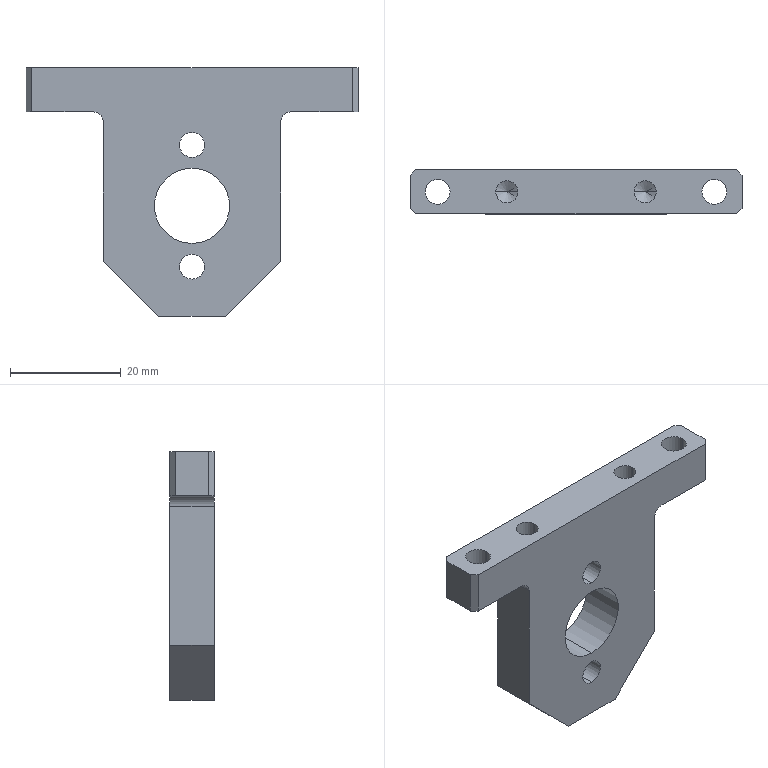Part | SolidWorks | features HoleWzd 3, Chamfer 2, Extrusion 1, ICE 1 | 1 solid | 42 faces | box 60 x 8 x 45 mm | volume 10317 mm3 | cylinder 20 | plane 18 | cone 4 | commonest cylinder face diameters 4.5 x8 4 x6 7.5 x4 13.6 x2
STEP:
#1=CARTESIAN_POINT('',(27.25,0.,0.));
#2=VERTEX_POINT('',#1);
#3=CARTESIAN_POINT('',(22.75,0.,0.));
#4=VERTEX_POINT('',#3);
#5=CARTESIAN_POINT('',(25.,0.,0.));
#6=DIRECTION('',(0.,0.,-1.));
#7=DIRECTION('',(-1.,0.,0.));
#8=AXIS2_PLACEMENT_3D('',#5,#6,#7);
#9=CIRCLE('',#8,2.25);
#10=EDGE_CURVE('',#2,#4,#9,.T.);
#11=ORIENTED_EDGE('',*,*,#10,.F.);
#12=CARTESIAN_POINT('',(27.25,0.,-8.));
#13=VERTEX_POINT('',#12);
#14=CARTESIAN_POINT('',(27.25,0.,-8.));
#15=DIRECTION('',(0.,0.,-1.));
#16=VECTOR('',#15,1000.);
#17=LINE('',#14,#16);
#18=EDGE_CURVE('',#2,#13,#17,.T.);
#19=ORIENTED_EDGE('',*,*,#18,.T.);
#20=CARTESIAN_POINT('',(22.75,0.,-8.));
#21=VERTEX_POINT('',#20);
#22=CARTESIAN_POINT('',(25.,0.,-8.));
#23=DIRECTION('',(0.,0.,-1.));
#24=DIRECTION('',(-1.,0.,0.));
#25=AXIS2_PLACEMENT_3D('',#22,#23,#24);
#26=CIRCLE('',#25,2.25);
#27=EDGE_CURVE('',#13,#21,#26,.T.);
#28=ORIENTED_EDGE('',*,*,#27,.T.);
#29=CARTESIAN_POINT('',(22.75,0.,-8.));
#30=DIRECTION('',(0.,0.,-1.));
#31=VECTOR('',#30,1000.);
#32=LINE('',#29,#31);
#33=EDGE_CURVE('',#4,#21,#32,.T.);
#34=ORIENTED_EDGE('',*,*,#33,.F.);
#35=EDGE_LOOP('',(#11,#19,#28,#34));
#36=FACE_OUTER_BOUND('',#35,.T.);
#37=CARTESIAN_POINT('',(25.,0.,-8.));
#38=DIRECTION('',(0.,0.,-1.));
#39=DIRECTION('',(-1.,0.,0.));
#40=AXIS2_PLACEMENT_3D('',#37,#38,#39);
#41=CYLINDRICAL_SURFACE('',#40,2.25);
#42=ADVANCED_FACE('',(#36),#41,.F.);
#43=CARTESIAN_POINT('',(-22.75,0.,0.));
#44=VERTEX_POINT('',#43);
#45=CARTESIAN_POINT('',(-27.25,0.,0.));
#46=VERTEX_POINT('',#45);
#47=CARTESIAN_POINT('',(-25.,0.,0.));
#48=DIRECTION('',(0.,0.,-1.));
#49=DIRECTION('',(-1.,0.,0.));
#50=AXIS2_PLACEMENT_3D('',#47,#48,#49);
#51=CIRCLE('',#50,2.25);
#52=EDGE_CURVE('',#44,#46,#51,.T.);
#53=ORIENTED_EDGE('',*,*,#52,.F.);
#54=CARTESIAN_POINT('',(-22.75,0.,-8.));
#55=VERTEX_POINT('',#54);
#56=CARTESIAN_POINT('',(-22.75,0.,-8.));
#57=DIRECTION('',(0.,0.,-1.));
#58=VECTOR('',#57,1000.);
#59=LINE('',#56,#58);
#60=EDGE_CURVE('',#44,#55,#59,.T.);
#61=ORIENTED_EDGE('',*,*,#60,.T.);
#62=CARTESIAN_POINT('',(-27.25,0.,-8.));
#63=VERTEX_POINT('',#62);
#64=CARTESIAN_POINT('',(-25.,0.,-8.));
#65=DIRECTION('',(0.,0.,-1.));
#66=DIRECTION('',(-1.,0.,0.));
#67=AXIS2_PLACEMENT_3D('',#64,#65,#66);
#68=CIRCLE('',#67,2.25);
#69=EDGE_CURVE('',#55,#63,#68,.T.);
#70=ORIENTED_EDGE('',*,*,#69,.T.);
#71=CARTESIAN_POINT('',(-27.25,0.,-8.));
#72=DIRECTION('',(0.,0.,-1.));
#73=VECTOR('',#72,1000.);
#74=LINE('',#71,#73);
#75=EDGE_CURVE('',#46,#63,#74,.T.);
#76=ORIENTED_EDGE('',*,*,#75,.F.);
#77=EDGE_LOOP('',(#53,#61,#70,#76));
#78=FACE_OUTER_BOUND('',#77,.T.);
#79=CARTESIAN_POINT('',(-25.,0.,-8.));
#80=DIRECTION('',(0.,0.,-1.));
#81=DIRECTION('',(-1.,0.,0.));
#82=AXIS2_PLACEMENT_3D('',#79,#80,#81);
#83=CYLINDRICAL_SURFACE('',#82,2.25);
#84=ADVANCED_FACE('',(#78),#83,.F.);
#85=CARTESIAN_POINT('',(-14.5,0.,-10.));
#86=VERTEX_POINT('',#85);
#87=CARTESIAN_POINT('',(-10.5,0.,-10.));
#88=VERTEX_POINT('',#87);
#89=CARTESIAN_POINT('',(-12.5,0.,-10.));
#90=DIRECTION('',(0.,0.,1.));
#91=DIRECTION('',(1.,0.,0.));
#92=AXIS2_PLACEMENT_3D('',#89,#90,#91);
#93=CIRCLE('',#92,2.);
#94=EDGE_CURVE('',#86,#88,#93,.T.);
#95=ORIENTED_EDGE('',*,*,#94,.F.);
#96=CARTESIAN_POINT('',(-14.5,0.,0.));
#97=VERTEX_POINT('',#96);
#98=CARTESIAN_POINT('',(-14.5,0.,0.));
#99=DIRECTION('',(0.,0.,1.));
#100=VECTOR('',#99,1000.);
#101=LINE('',#98,#100);
#102=EDGE_CURVE('',#86,#97,#101,.T.);
#103=ORIENTED_EDGE('',*,*,#102,.T.);
#104=CARTESIAN_POINT('',(-10.5,0.,0.));
#105=VERTEX_POINT('',#104);
#106=CARTESIAN_POINT('',(-12.5,0.,0.));
#107=DIRECTION('',(0.,0.,1.));
#108=DIRECTION('',(1.,0.,0.));
#109=AXIS2_PLACEMENT_3D('',#106,#107,#108);
#110=CIRCLE('',#109,2.);
#111=EDGE_CURVE('',#97,#105,#110,.T.);
#112=ORIENTED_EDGE('',*,*,#111,.T.);
#113=CARTESIAN_POINT('',(-10.5,0.,0.));
#114=DIRECTION('',(0.,0.,1.));
#115=VECTOR('',#114,1000.);
#116=LINE('',#113,#115);
#117=EDGE_CURVE('',#88,#105,#116,.T.);
#118=ORIENTED_EDGE('',*,*,#117,.F.);
#119=EDGE_LOOP('',(#95,#103,#112,#118));
#120=FACE_OUTER_BOUND('',#119,.T.);
#121=CARTESIAN_POINT('',(-12.5,0.,0.));
#122=DIRECTION('',(0.,0.,1.));
#123=DIRECTION('',(1.,0.,0.));
#124=AXIS2_PLACEMENT_3D('',#121,#122,#123);
#125=CYLINDRICAL_SURFACE('',#124,2.);
#126=ADVANCED_FACE('',(#120),#125,.F.);
#127=CARTESIAN_POINT('',(-12.5,0.,-11.202));
#128=VERTEX_POINT('',#127);
#129=CARTESIAN_POINT('',(-10.5,0.,-10.));
#130=DIRECTION('',(0.8572,0.,0.515));
#131=VECTOR('',#130,1000.);
#132=LINE('',#129,#131);
#133=EDGE_CURVE('',#128,#88,#132,.T.);
#134=ORIENTED_EDGE('',*,*,#133,.F.);
#135=CARTESIAN_POINT('',(-14.5,0.,-10.));
#136=DIRECTION('',(-0.8572,0.,0.515));
#137=VECTOR('',#136,1000.);
#138=LINE('',#135,#137);
#139=EDGE_CURVE('',#128,#86,#138,.T.);
#140=ORIENTED_EDGE('',*,*,#139,.T.);
#141=ORIENTED_EDGE('',*,*,#94,.T.);
#142=EDGE_LOOP('',(#134,#140,#141));
#143=FACE_OUTER_BOUND('',#142,.T.);
#144=CARTESIAN_POINT('',(-12.5,0.,-10.));
#145=DIRECTION('',(0.,0.,1.));
#146=DIRECTION('',(1.,0.,0.));
#147=AXIS2_PLACEMENT_3D('',#144,#145,#146);
#148=CONICAL_SURFACE('',#147,2.,1.03);
#149=ADVANCED_FACE('',(#143),#148,.F.);
#150=CARTESIAN_POINT('',(10.5,0.,-10.));
#151=VERTEX_POINT('',#150);
#152=CARTESIAN_POINT('',(14.5,0.,-10.));
#153=VERTEX_POINT('',#152);
#154=CARTESIAN_POINT('',(12.5,0.,-10.));
#155=DIRECTION('',(0.,0.,1.));
#156=DIRECTION('',(1.,0.,0.));
#157=AXIS2_PLACEMENT_3D('',#154,#155,#156);
#158=CIRCLE('',#157,2.);
#159=EDGE_CURVE('',#151,#153,#158,.T.);
#160=ORIENTED_EDGE('',*,*,#159,.F.);
#161=CARTESIAN_POINT('',(10.5,0.,0.));
#162=VERTEX_POINT('',#161);
#163=CARTESIAN_POINT('',(10.5,0.,0.));
#164=DIRECTION('',(0.,0.,1.));
#165=VECTOR('',#164,1000.);
#166=LINE('',#163,#165);
#167=EDGE_CURVE('',#151,#162,#166,.T.);
#168=ORIENTED_EDGE('',*,*,#167,.T.);
#169=CARTESIAN_POINT('',(14.5,0.,0.));
#170=VERTEX_POINT('',#169);
#171=CARTESIAN_POINT('',(12.5,0.,0.));
#172=DIRECTION('',(0.,0.,1.));
#173=DIRECTION('',(1.,0.,0.));
#174=AXIS2_PLACEMENT_3D('',#171,#172,#173);
#175=CIRCLE('',#174,2.);
#176=EDGE_CURVE('',#162,#170,#175,.T.);
#177=ORIENTED_EDGE('',*,*,#176,.T.);
#178=CARTESIAN_POINT('',(14.5,0.,0.));
#179=DIRECTION('',(0.,0.,1.));
#180=VECTOR('',#179,1000.);
#181=LINE('',#178,#180);
#182=EDGE_CURVE('',#153,#170,#181,.T.);
#183=ORIENTED_EDGE('',*,*,#182,.F.);
#184=EDGE_LOOP('',(#160,#168,#177,#183));
#185=FACE_OUTER_BOUND('',#184,.T.);
#186=CARTESIAN_POINT('',(12.5,0.,0.));
#187=DIRECTION('',(0.,0.,1.));
#188=DIRECTION('',(1.,0.,0.));
#189=AXIS2_PLACEMENT_3D('',#186,#187,#188);
#190=CYLINDRICAL_SURFACE('',#189,2.);
#191=ADVANCED_FACE('',(#185),#190,.F.);
#192=CARTESIAN_POINT('',(12.5,0.,-11.202));
#193=VERTEX_POINT('',#192);
#194=CARTESIAN_POINT('',(14.5,0.,-10.));
#195=DIRECTION('',(0.8572,0.,0.515));
#196=VECTOR('',#195,1000.);
#197=LINE('',#194,#196);
#198=EDGE_CURVE('',#193,#153,#197,.T.);
#199=ORIENTED_EDGE('',*,*,#198,.F.);
#200=CARTESIAN_POINT('',(10.5,0.,-10.));
#201=DIRECTION('',(-0.8572,0.,0.515));
#202=VECTOR('',#201,1000.);
#203=LINE('',#200,#202);
#204=EDGE_CURVE('',#193,#151,#203,.T.);
#205=ORIENTED_EDGE('',*,*,#204,.T.);
#206=ORIENTED_EDGE('',*,*,#159,.T.);
#207=EDGE_LOOP('',(#199,#205,#206));
#208=FACE_OUTER_BOUND('',#207,.T.);
#209=CARTESIAN_POINT('',(12.5,0.,-10.));
#210=DIRECTION('',(0.,0.,1.));
#211=DIRECTION('',(1.,0.,0.));
#212=AXIS2_PLACEMENT_3D('',#209,#210,#211);
#213=CONICAL_SURFACE('',#212,2.,1.03);
#214=ADVANCED_FACE('',(#208),#213,.F.);
#215=CARTESIAN_POINT('',(0.,-0.6,-39.75));
#216=VERTEX_POINT('',#215);
#217=CARTESIAN_POINT('',(0.,-0.6,-32.25));
#218=VERTEX_POINT('',#217);
#219=CARTESIAN_POINT('',(0.,-0.6,-36.));
#220=DIRECTION('',(0.,1.,0.));
#221=DIRECTION('',(0.,0.,1.));
#222=AXIS2_PLACEMENT_3D('',#219,#220,#221);
#223=CIRCLE('',#222,3.75);
#224=EDGE_CURVE('',#216,#218,#223,.T.);
#225=ORIENTED_EDGE('',*,*,#224,.F.);
#226=CARTESIAN_POINT('',(0.,4.,-39.75));
#227=VERTEX_POINT('',#226);
#228=CARTESIAN_POINT('',(0.,4.,-39.75));
#229=DIRECTION('',(0.,1.,0.));
#230=VECTOR('',#229,1000.);
#231=LINE('',#228,#230);
#232=EDGE_CURVE('',#216,#227,#231,.T.);
#233=ORIENTED_EDGE('',*,*,#232,.T.);
#234=CARTESIAN_POINT('',(0.,4.,-32.25));
#235=VERTEX_POINT('',#234);
#236=CARTESIAN_POINT('',(0.,4.,-36.));
#237=DIRECTION('',(0.,1.,0.));
#238=DIRECTION('',(0.,0.,1.));
#239=AXIS2_PLACEMENT_3D('',#236,#237,#238);
#240=CIRCLE('',#239,3.75);
#241=EDGE_CURVE('',#227,#235,#240,.T.);
#242=ORIENTED_EDGE('',*,*,#241,.T.);
#243=CARTESIAN_POINT('',(0.,4.,-32.25));
#244=DIRECTION('',(0.,1.,0.));
#245=VECTOR('',#244,1000.);
#246=LINE('',#243,#245);
#247=EDGE_CURVE('',#218,#235,#246,.T.);
#248=ORIENTED_EDGE('',*,*,#247,.F.);
#249=EDGE_LOOP('',(#225,#233,#242,#248));
#250=FACE_OUTER_BOUND('',#249,.T.);
#251=CARTESIAN_POINT('',(0.,4.,-36.));
#252=DIRECTION('',(0.,1.,0.));
#253=DIRECTION('',(0.,0.,1.));
#254=AXIS2_PLACEMENT_3D('',#251,#252,#253);
#255=CYLINDRICAL_SURFACE('',#254,3.75);
#256=ADVANCED_FACE('',(#250),#255,.F.);
#257=CARTESIAN_POINT('',(0.,-4.,-33.75));
#258=VERTEX_POINT('',#257);
#259=CARTESIAN_POINT('',(0.,-4.,-38.25));
#260=VERTEX_POINT('',#259);
#261=CARTESIAN_POINT('',(0.,-4.,-36.));
#262=DIRECTION('',(0.,-1.,0.));
#263=DIRECTION('',(0.,0.,-1.));
#264=AXIS2_PLACEMENT_3D('',#261,#262,#263);
#265=CIRCLE('',#264,2.25);
#266=EDGE_CURVE('',#258,#260,#265,.T.);
#267=ORIENTED_EDGE('',*,*,#266,.T.);
#268=CARTESIAN_POINT('',(0.,-0.6,-38.25));
#269=VERTEX_POINT('',#268);
#270=CARTESIAN_POINT('',(0.,4.,-38.25));
#271=DIRECTION('',(0.,1.,0.));
#272=VECTOR('',#271,1000.);
#273=LINE('',#270,#272);
#274=EDGE_CURVE('',#260,#269,#273,.T.);
#275=ORIENTED_EDGE('',*,*,#274,.T.);
#276=CARTESIAN_POINT('',(0.,-0.6,-33.75));
#277=VERTEX_POINT('',#276);
#278=CARTESIAN_POINT('',(0.,-0.6,-36.));
#279=DIRECTION('',(0.,1.,0.));
#280=DIRECTION('',(0.,0.,1.));
#281=AXIS2_PLACEMENT_3D('',#278,#279,#280);
#282=CIRCLE('',#281,2.25);
#283=EDGE_CURVE('',#269,#277,#282,.T.);
#284=ORIENTED_EDGE('',*,*,#283,.T.);
#285=CARTESIAN_POINT('',(0.,4.,-33.75));
#286=DIRECTION('',(0.,1.,0.));
#287=VECTOR('',#286,1000.);
#288=LINE('',#285,#287);
#289=EDGE_CURVE('',#258,#277,#288,.T.);
#290=ORIENTED_EDGE('',*,*,#289,.F.);
#291=EDGE_LOOP('',(#267,#275,#284,#290));
#292=FACE_OUTER_BOUND('',#291,.T.);
#293=CARTESIAN_POINT('',(0.,4.,-36.));
#294=DIRECTION('',(0.,1.,0.));
#295=DIRECTION('',(0.,0.,1.));
#296=AXIS2_PLACEMENT_3D('',#293,#294,#295);
#297=CYLINDRICAL_SURFACE('',#296,2.25);
#298=ADVANCED_FACE('',(#292),#297,.F.);
#299=CARTESIAN_POINT('',(0.,-0.6,-17.75));
#300=VERTEX_POINT('',#299);
#301=CARTESIAN_POINT('',(0.,-0.6,-10.25));
#302=VERTEX_POINT('',#301);
#303=CARTESIAN_POINT('',(0.,-0.6,-14.));
#304=DIRECTION('',(0.,1.,0.));
#305=DIRECTION('',(0.,0.,1.));
#306=AXIS2_PLACEMENT_3D('',#303,#304,#305);
#307=CIRCLE('',#306,3.75);
#308=EDGE_CURVE('',#300,#302,#307,.T.);
#309=ORIENTED_EDGE('',*,*,#308,.F.);
#310=CARTESIAN_POINT('',(0.,4.,-17.75));
#311=VERTEX_POINT('',#310);
#312=CARTESIAN_POINT('',(0.,4.,-17.75));
#313=DIRECTION('',(0.,1.,0.));
#314=VECTOR('',#313,1000.);
#315=LINE('',#312,#314);
#316=EDGE_CURVE('',#300,#311,#315,.T.);
#317=ORIENTED_EDGE('',*,*,#316,.T.);
#318=CARTESIAN_POINT('',(0.,4.,-10.25));
#319=VERTEX_POINT('',#318);
#320=CARTESIAN_POINT('',(0.,4.,-14.));
#321=DIRECTION('',(0.,1.,0.));
#322=DIRECTION('',(0.,0.,1.));
#323=AXIS2_PLACEMENT_3D('',#320,#321,#322);
#324=CIRCLE('',#323,3.75);
#325=EDGE_CURVE('',#311,#319,#324,.T.);
#326=ORIENTED_EDGE('',*,*,#325,.T.);
#327=CARTESIAN_POINT('',(0.,4.,-10.25));
#328=DIRECTION('',(0.,1.,0.));
#329=VECTOR('',#328,1000.);
#330=LINE('',#327,#329);
#331=EDGE_CURVE('',#302,#319,#330,.T.);
#332=ORIENTED_EDGE('',*,*,#331,.F.);
#333=EDGE_LOOP('',(#309,#317,#326,#332));
#334=FACE_OUTER_BOUND('',#333,.T.);
#335=CARTESIAN_POINT('',(0.,4.,-14.));
#336=DIRECTION('',(0.,1.,0.));
#337=DIRECTION('',(0.,0.,1.));
#338=AXIS2_PLACEMENT_3D('',#335,#336,#337);
#339=CYLINDRICAL_SURFACE('',#338,3.75);
#340=ADVANCED_FACE('',(#334),#339,.F.);
#341=CARTESIAN_POINT('',(0.,-4.,-11.75));
#342=VERTEX_POINT('',#341);
#343=CARTESIAN_POINT('',(0.,-4.,-16.25));
#344=VERTEX_POINT('',#343);
#345=CARTESIAN_POINT('',(0.,-4.,-14.));
#346=DIRECTION('',(0.,-1.,0.));
#347=DIRECTION('',(0.,0.,-1.));
#348=AXIS2_PLACEMENT_3D('',#345,#346,#347);
#349=CIRCLE('',#348,2.25);
#350=EDGE_CURVE('',#342,#344,#349,.T.);
#351=ORIENTED_EDGE('',*,*,#350,.T.);
#352=CARTESIAN_POINT('',(0.,-0.6,-16.25));
#353=VERTEX_POINT('',#352);
#354=CARTESIAN_POINT('',(0.,4.,-16.25));
#355=DIRECTION('',(0.,1.,0.));
#356=VECTOR('',#355,1000.);
#357=LINE('',#354,#356);
#358=EDGE_CURVE('',#344,#353,#357,.T.);
#359=ORIENTED_EDGE('',*,*,#358,.T.);
#360=CARTESIAN_POINT('',(0.,-0.6,-11.75));
#361=VERTEX_POINT('',#360);
#362=CARTESIAN_POINT('',(0.,-0.6,-14.));
#363=DIRECTION('',(0.,1.,0.));
#364=DIRECTION('',(0.,0.,1.));
#365=AXIS2_PLACEMENT_3D('',#362,#363,#364);
#366=CIRCLE('',#365,2.25);
#367=EDGE_CURVE('',#353,#361,#366,.T.);
#368=ORIENTED_EDGE('',*,*,#367,.T.);
#369=CARTESIAN_POINT('',(0.,4.,-11.75));
#370=DIRECTION('',(0.,1.,0.));
#371=VECTOR('',#370,1000.);
#372=LINE('',#369,#371);
#373=EDGE_CURVE('',#342,#361,#372,.T.);
#374=ORIENTED_EDGE('',*,*,#373,.F.);
#375=EDGE_LOOP('',(#351,#359,#368,#374));
#376=FACE_OUTER_BOUND('',#375,.T.);
#377=CARTESIAN_POINT('',(0.,4.,-14.));
#378=DIRECTION('',(0.,1.,0.));
#379=DIRECTION('',(0.,0.,1.));
#380=AXIS2_PLACEMENT_3D('',#377,#378,#379);
#381=CYLINDRICAL_SURFACE('',#380,2.25);
#382=ADVANCED_FACE('',(#376),#381,.F.);
#383=CARTESIAN_POINT('',(0.,-4.,-31.8));
#384=VERTEX_POINT('',#383);
#385=CARTESIAN_POINT('',(0.,-4.,-18.2));
#386=VERTEX_POINT('',#385);
#387=CARTESIAN_POINT('',(0.,-4.,-25.));
#388=DIRECTION('',(0.,1.,0.));
#389=DIRECTION('',(0.,0.,-1.));
#390=AXIS2_PLACEMENT_3D('',#387,#388,#389);
#391=CIRCLE('',#390,6.8);
#392=EDGE_CURVE('',#384,#386,#391,.T.);
#393=ORIENTED_EDGE('',*,*,#392,.F.);
#394=CARTESIAN_POINT('',(0.,4.,-31.8));
#395=VERTEX_POINT('',#394);
#396=CARTESIAN_POINT('',(0.,-4.001,-31.8));
#397=DIRECTION('',(0.,1.,0.));
#398=VECTOR('',#397,1000.);
#399=LINE('',#396,#398);
#400=EDGE_CURVE('',#384,#395,#399,.T.);
#401=ORIENTED_EDGE('',*,*,#400,.T.);
#402=CARTESIAN_POINT('',(0.,4.,-18.2));
#403=VERTEX_POINT('',#402);
#404=CARTESIAN_POINT('',(0.,4.,-25.));
#405=DIRECTION('',(0.,1.,0.));
#406=DIRECTION('',(0.,0.,1.));
#407=AXIS2_PLACEMENT_3D('',#404,#405,#406);
#408=CIRCLE('',#407,6.8);
#409=EDGE_CURVE('',#395,#403,#408,.T.);
#410=ORIENTED_EDGE('',*,*,#409,.T.);
#411=CARTESIAN_POINT('',(0.,-4.001,-18.2));
#412=DIRECTION('',(0.,1.,0.));
#413=VECTOR('',#412,1000.);
#414=LINE('',#411,#413);
#415=EDGE_CURVE('',#386,#403,#414,.T.);
#416=ORIENTED_EDGE('',*,*,#415,.F.);
#417=EDGE_LOOP('',(#393,#401,#410,#416));
#418=FACE_OUTER_BOUND('',#417,.T.);
#419=CARTESIAN_POINT('',(0.,-4.001,-25.));
#420=DIRECTION('',(0.,1.,0.));
#421=DIRECTION('',(0.,0.,1.));
#422=AXIS2_PLACEMENT_3D('',#419,#420,#421);
#423=CYLINDRICAL_SURFACE('',#422,6.8);
#424=ADVANCED_FACE('',(#418),#423,.F.);
#425=CARTESIAN_POINT('',(30.,3.,-8.));
#426=VERTEX_POINT('',#425);
#427=CARTESIAN_POINT('',(30.,-3.,-8.));
#428=VERTEX_POINT('',#427);
#429=CARTESIAN_POINT('',(30.,4.,-8.));
#430=DIRECTION('',(0.,-1.,0.));
#431=VECTOR('',#430,1000.);
#432=LINE('',#429,#431);
#433=EDGE_CURVE('',#426,#428,#432,.T.);
#434=ORIENTED_EDGE('',*,*,#433,.T.);
#435=CARTESIAN_POINT('',(29.,-4.,-8.));
#436=VERTEX_POINT('',#435);
#437=CARTESIAN_POINT('',(30.,-3.,-8.));
#438=DIRECTION('',(-0.7071,-0.7071,0.));
#439=VECTOR('',#438,1000.);
#440=LINE('',#437,#439);
#441=EDGE_CURVE('',#428,#436,#440,.T.);
#442=ORIENTED_EDGE('',*,*,#441,.T.);
#443=CARTESIAN_POINT('',(18.,-4.,-8.));
#444=VERTEX_POINT('',#443);
#445=CARTESIAN_POINT('',(30.,-4.,-8.));
#446=DIRECTION('',(-1.,0.,0.));
#447=VECTOR('',#446,1000.);
#448=LINE('',#445,#447);
#449=EDGE_CURVE('',#436,#444,#448,.T.);
#450=ORIENTED_EDGE('',*,*,#449,.T.);
#451=CARTESIAN_POINT('',(18.,4.,-8.));
#452=VERTEX_POINT('',#451);
#453=CARTESIAN_POINT('',(18.,4.,-8.));
#454=DIRECTION('',(0.,-1.,0.));
#455=VECTOR('',#454,1000.);
#456=LINE('',#453,#455);
#457=EDGE_CURVE('',#452,#444,#456,.T.);
#458=ORIENTED_EDGE('',*,*,#457,.F.);
#459=CARTESIAN_POINT('',(29.,4.,-8.));
#460=VERTEX_POINT('',#459);
#461=CARTESIAN_POINT('',(30.,4.,-8.));
#462=DIRECTION('',(-1.,0.,0.));
#463=VECTOR('',#462,1000.);
#464=LINE('',#461,#463);
#465=EDGE_CURVE('',#460,#452,#464,.T.);
#466=ORIENTED_EDGE('',*,*,#465,.F.);
#467=CARTESIAN_POINT('',(29.,4.,-8.));
#468=DIRECTION('',(0.7071,-0.7071,0.));
#469=VECTOR('',#468,1000.);
#470=LINE('',#467,#469);
#471=EDGE_CURVE('',#460,#426,#470,.T.);
#472=ORIENTED_EDGE('',*,*,#471,.T.);
#473=EDGE_LOOP('',(#434,#442,#450,#458,#466,#472));
#474=FACE_OUTER_BOUND('',#473,.T.);
#475=CARTESIAN_POINT('',(25.,0.,-8.));
#476=DIRECTION('',(0.,0.,-1.));
#477=DIRECTION('',(-1.,0.,0.));
#478=AXIS2_PLACEMENT_3D('',#475,#476,#477);
#479=CIRCLE('',#478,2.25);
#480=EDGE_CURVE('',#21,#13,#479,.T.);
#481=ORIENTED_EDGE('',*,*,#480,.F.);
#482=ORIENTED_EDGE('',*,*,#27,.F.);
#483=EDGE_LOOP('',(#481,#482));
#484=FACE_BOUND('',#483,.T.);
#485=CARTESIAN_POINT('',(30.,4.,-8.));
#486=DIRECTION('',(0.,0.,1.));
#487=DIRECTION('',(1.,0.,0.));
#488=AXIS2_PLACEMENT_3D('',#485,#486,#487);
#489=PLANE('',#488);
#490=ADVANCED_FACE('',(#474,#484),#489,.F.);
#491=CARTESIAN_POINT('',(-18.,-4.,-8.));
#492=VERTEX_POINT('',#491);
#493=CARTESIAN_POINT('',(-29.,-4.,-8.));
#494=VERTEX_POINT('',#493);
#495=CARTESIAN_POINT('',(-18.,-4.,-8.));
#496=DIRECTION('',(-1.,0.,0.));
#497=VECTOR('',#496,1000.);
#498=LINE('',#495,#497);
#499=EDGE_CURVE('',#492,#494,#498,.T.);
#500=ORIENTED_EDGE('',*,*,#499,.T.);
#501=CARTESIAN_POINT('',(-30.,-3.,-8.));
#502=VERTEX_POINT('',#501);
#503=CARTESIAN_POINT('',(-30.,-3.,-8.));
#504=DIRECTION('',(-0.7071,0.7071,0.));
#505=VECTOR('',#504,1000.);
#506=LINE('',#503,#505);
#507=EDGE_CURVE('',#494,#502,#506,.T.);
#508=ORIENTED_EDGE('',*,*,#507,.T.);
#509=CARTESIAN_POINT('',(-30.,3.,-8.));
#510=VERTEX_POINT('',#509);
#511=CARTESIAN_POINT('',(-30.,4.,-8.));
#512=DIRECTION('',(0.,-1.,0.));
#513=VECTOR('',#512,1000.);
#514=LINE('',#511,#513);
#515=EDGE_CURVE('',#510,#502,#514,.T.);
#516=ORIENTED_EDGE('',*,*,#515,.F.);
#517=CARTESIAN_POINT('',(-29.,4.,-8.));
#518=VERTEX_POINT('',#517);
#519=CARTESIAN_POINT('',(-29.,4.,-8.));
#520=DIRECTION('',(0.7071,0.7071,0.));
#521=VECTOR('',#520,1000.);
#522=LINE('',#519,#521);
#523=EDGE_CURVE('',#510,#518,#522,.T.);
#524=ORIENTED_EDGE('',*,*,#523,.T.);
#525=CARTESIAN_POINT('',(-18.,4.,-8.));
#526=VERTEX_POINT('',#525);
#527=CARTESIAN_POINT('',(-18.,4.,-8.));
#528=DIRECTION('',(-1.,0.,0.));
#529=VECTOR('',#528,1000.);
#530=LINE('',#527,#529);
#531=EDGE_CURVE('',#526,#518,#530,.T.);
#532=ORIENTED_EDGE('',*,*,#531,.F.);
#533=CARTESIAN_POINT('',(-18.,4.,-8.));
#534=DIRECTION('',(0.,-1.,0.));
#535=VECTOR('',#534,1000.);
#536=LINE('',#533,#535);
#537=EDGE_CURVE('',#526,#492,#536,.T.);
#538=ORIENTED_EDGE('',*,*,#537,.T.);
#539=EDGE_LOOP('',(#500,#508,#516,#524,#532,#538));
#540=FACE_OUTER_BOUND('',#539,.T.);
#541=CARTESIAN_POINT('',(-25.,0.,-8.));
#542=DIRECTION('',(0.,0.,-1.));
#543=DIRECTION('',(-1.,0.,0.));
#544=AXIS2_PLACEMENT_3D('',#541,#542,#543);
#545=CIRCLE('',#544,2.25);
#546=EDGE_CURVE('',#63,#55,#545,.T.);
#547=ORIENTED_EDGE('',*,*,#546,.F.);
#548=ORIENTED_EDGE('',*,*,#69,.F.);
#549=EDGE_LOOP('',(#547,#548));
#550=FACE_BOUND('',#549,.T.);
#551=CARTESIAN_POINT('',(-18.,4.,-8.));
#552=DIRECTION('',(0.,0.,1.));
#553=DIRECTION('',(1.,0.,0.));
#554=AXIS2_PLACEMENT_3D('',#551,#552,#553);
#555=PLANE('',#554);
#556=ADVANCED_FACE('',(#540,#550),#555,.F.);
#557=ORIENTED_EDGE('',*,*,#515,.T.);
#558=CARTESIAN_POINT('',(-30.,-3.,0.));
#559=VERTEX_POINT('',#558);
#560=CARTESIAN_POINT('',(-30.,-3.,0.));
#561=DIRECTION('',(0.,0.,1.));
#562=VECTOR('',#561,1000.);
#563=LINE('',#560,#562);
#564=EDGE_CURVE('',#502,#559,#563,.T.);
#565=ORIENTED_EDGE('',*,*,#564,.T.);
#566=CARTESIAN_POINT('',(-30.,3.,0.));
#567=VERTEX_POINT('',#566);
#568=CARTESIAN_POINT('',(-30.,4.,0.));
#569=DIRECTION('',(0.,-1.,0.));
#570=VECTOR('',#569,1000.);
#571=LINE('',#568,#570);
#572=EDGE_CURVE('',#567,#559,#571,.T.);
#573=ORIENTED_EDGE('',*,*,#572,.F.);
#574=CARTESIAN_POINT('',(-30.,3.,-8.));
#575=DIRECTION('',(0.,0.,-1.));
#576=VECTOR('',#575,1000.);
#577=LINE('',#574,#576);
#578=EDGE_CURVE('',#567,#510,#577,.T.);
#579=ORIENTED_EDGE('',*,*,#578,.T.);
#580=EDGE_LOOP('',(#557,#565,#573,#579));
#581=FACE_OUTER_BOUND('',#580,.T.);
#582=CARTESIAN_POINT('',(-30.,4.,-8.));
#583=DIRECTION('',(1.,0.,0.));
#584=DIRECTION('',(0.,0.,-1.));
#585=AXIS2_PLACEMENT_3D('',#582,#583,#584);
#586=PLANE('',#585);
#587=ADVANCED_FACE('',(#581),#586,.F.);
#588=CARTESIAN_POINT('',(25.,0.,0.));
#589=DIRECTION('',(0.,0.,-1.));
#590=DIRECTION('',(-1.,0.,0.));
#591=AXIS2_PLACEMENT_3D('',#588,#589,#590);
#592=CIRCLE('',#591,2.25);
#593=EDGE_CURVE('',#4,#2,#592,.T.);
#594=ORIENTED_EDGE('',*,*,#593,.T.);
#595=ORIENTED_EDGE('',*,*,#10,.T.);
#596=EDGE_LOOP('',(#594,#595));
#597=FACE_BOUND('',#596,.T.);
#598=CARTESIAN_POINT('',(-25.,0.,0.));
#599=DIRECTION('',(0.,0.,-1.));
#600=DIRECTION('',(-1.,0.,0.));
#601=AXIS2_PLACEMENT_3D('',#598,#599,#600);
#602=CIRCLE('',#601,2.25);
#603=EDGE_CURVE('',#46,#44,#602,.T.);
#604=ORIENTED_EDGE('',*,*,#603,.T.);
#605=ORIENTED_EDGE('',*,*,#52,.T.);
#606=EDGE_LOOP('',(#604,#605));
#607=FACE_BOUND('',#606,.T.);
#608=CARTESIAN_POINT('',(-12.5,0.,0.));
#609=DIRECTION('',(0.,0.,1.));
#610=DIRECTION('',(1.,0.,0.));
#611=AXIS2_PLACEMENT_3D('',#608,#609,#610);
#612=CIRCLE('',#611,2.);
#613=EDGE_CURVE('',#105,#97,#612,.T.);
#614=ORIENTED_EDGE('',*,*,#613,.F.);
#615=ORIENTED_EDGE('',*,*,#111,.F.);
#616=EDGE_LOOP('',(#614,#615));
#617=FACE_BOUND('',#616,.T.);
#618=CARTESIAN_POINT('',(12.5,0.,0.));
#619=DIRECTION('',(0.,0.,1.));
#620=DIRECTION('',(1.,0.,0.));
#621=AXIS2_PLACEMENT_3D('',#618,#619,#620);
#622=CIRCLE('',#621,2.);
#623=EDGE_CURVE('',#170,#162,#622,.T.);
#624=ORIENTED_EDGE('',*,*,#623,.F.);
#625=ORIENTED_EDGE('',*,*,#176,.F.);
#626=EDGE_LOOP('',(#624,#625));
#627=FACE_BOUND('',#626,.T.);
#628=CARTESIAN_POINT('',(-29.,-4.,0.));
#629=VERTEX_POINT('',#628);
#630=CARTESIAN_POINT('',(29.,-4.,0.));
#631=VERTEX_POINT('',#630);
#632=CARTESIAN_POINT('',(-30.,-4.,0.));
#633=DIRECTION('',(1.,0.,0.));
#634=VECTOR('',#633,1000.);
#635=LINE('',#632,#634);
#636=EDGE_CURVE('',#629,#631,#635,.T.);
#637=ORIENTED_EDGE('',*,*,#636,.T.);
#638=CARTESIAN_POINT('',(30.,-3.,0.));
#639=VERTEX_POINT('',#638);
#640=CARTESIAN_POINT('',(30.,-3.,0.));
#641=DIRECTION('',(0.7071,0.7071,0.));
#642=VECTOR('',#641,1000.);
#643=LINE('',#640,#642);
#644=EDGE_CURVE('',#631,#639,#643,.T.);
#645=ORIENTED_EDGE('',*,*,#644,.T.);
#646=CARTESIAN_POINT('',(30.,3.,0.));
#647=VERTEX_POINT('',#646);
#648=CARTESIAN_POINT('',(30.,4.,0.));
#649=DIRECTION('',(0.,-1.,0.));
#650=VECTOR('',#649,1000.);
#651=LINE('',#648,#650);
#652=EDGE_CURVE('',#647,#639,#651,.T.);
#653=ORIENTED_EDGE('',*,*,#652,.F.);
#654=CARTESIAN_POINT('',(29.,4.,0.));
#655=VERTEX_POINT('',#654);
#656=CARTESIAN_POINT('',(29.,4.,0.));
#657=DIRECTION('',(-0.7071,0.7071,0.));
#658=VECTOR('',#657,1000.);
#659=LINE('',#656,#658);
#660=EDGE_CURVE('',#647,#655,#659,.T.);
#661=ORIENTED_EDGE('',*,*,#660,.T.);
#662=CARTESIAN_POINT('',(-29.,4.,0.));
#663=VERTEX_POINT('',#662);
#664=CARTESIAN_POINT('',(-30.,4.,0.));
#665=DIRECTION('',(1.,0.,0.));
#666=VECTOR('',#665,1000.);
#667=LINE('',#664,#666);
#668=EDGE_CURVE('',#663,#655,#667,.T.);
#669=ORIENTED_EDGE('',*,*,#668,.F.);
#670=CARTESIAN_POINT('',(-29.,4.,0.));
#671=DIRECTION('',(-0.7071,-0.7071,0.));
#672=VECTOR('',#671,1000.);
#673=LINE('',#670,#672);
#674=EDGE_CURVE('',#663,#567,#673,.T.);
#675=ORIENTED_EDGE('',*,*,#674,.T.);
#676=ORIENTED_EDGE('',*,*,#572,.T.);
#677=CARTESIAN_POINT('',(-30.,-3.,0.));
#678=DIRECTION('',(0.7071,-0.7071,0.));
#679=VECTOR('',#678,1000.);
#680=LINE('',#677,#679);
#681=EDGE_CURVE('',#559,#629,#680,.T.);
#682=ORIENTED_EDGE('',*,*,#681,.T.);
#683=EDGE_LOOP('',(#637,#645,#653,#661,#669,#675,#676,#682));
#684=FACE_OUTER_BOUND('',#683,.T.);
#685=CARTESIAN_POINT('',(-30.,4.,0.));
#686=DIRECTION('',(0.,0.,-1.));
#687=DIRECTION('',(-1.,0.,0.));
#688=AXIS2_PLACEMENT_3D('',#685,#686,#687);
#689=PLANE('',#688);
#690=ADVANCED_FACE('',(#597,#607,#617,#627,#684),#689,.F.);
#691=ORIENTED_EDGE('',*,*,#652,.T.);
#692=CARTESIAN_POINT('',(30.,-3.,-8.));
#693=DIRECTION('',(0.,0.,-1.));
#694=VECTOR('',#693,1000.);
#695=LINE('',#692,#694);
#696=EDGE_CURVE('',#639,#428,#695,.T.);
#697=ORIENTED_EDGE('',*,*,#696,.T.);
#698=ORIENTED_EDGE('',*,*,#433,.F.);
#699=CARTESIAN_POINT('',(30.,3.,0.));
#700=DIRECTION('',(0.,0.,1.));
#701=VECTOR('',#700,1000.);
#702=LINE('',#699,#701);
#703=EDGE_CURVE('',#426,#647,#702,.T.);
#704=ORIENTED_EDGE('',*,*,#703,.T.);
#705=EDGE_LOOP('',(#691,#697,#698,#704));
#706=FACE_OUTER_BOUND('',#705,.T.);
#707=CARTESIAN_POINT('',(30.,4.,0.));
#708=DIRECTION('',(-1.,0.,0.));
#709=DIRECTION('',(0.,0.,1.));
#710=AXIS2_PLACEMENT_3D('',#707,#708,#709);
#711=PLANE('',#710);
#712=ADVANCED_FACE('',(#706),#711,.F.);
#713=CARTESIAN_POINT('',(16.,-4.,-10.));
#714=VERTEX_POINT('',#713);
#715=CARTESIAN_POINT('',(18.,-4.,-10.));
#716=DIRECTION('',(0.,-1.,0.));
#717=DIRECTION('',(0.,0.,-1.));
#718=AXIS2_PLACEMENT_3D('',#715,#716,#717);
#719=CIRCLE('',#718,2.);
#720=EDGE_CURVE('',#444,#714,#719,.T.);
#721=ORIENTED_EDGE('',*,*,#720,.T.);
#722=CARTESIAN_POINT('',(16.,4.,-10.));
#723=VERTEX_POINT('',#722);
#724=CARTESIAN_POINT('',(16.,4.,-10.));
#725=DIRECTION('',(0.,-1.,0.));
#726=VECTOR('',#725,1000.);
#727=LINE('',#724,#726);
#728=EDGE_CURVE('',#723,#714,#727,.T.);
#729=ORIENTED_EDGE('',*,*,#728,.F.);
#730=CARTESIAN_POINT('',(18.,4.,-10.));
#731=DIRECTION('',(0.,-1.,0.));
#732=DIRECTION('',(0.,0.,-1.));
#733=AXIS2_PLACEMENT_3D('',#730,#731,#732);
#734=CIRCLE('',#733,2.);
#735=EDGE_CURVE('',#452,#723,#734,.T.);
#736=ORIENTED_EDGE('',*,*,#735,.F.);
#737=ORIENTED_EDGE('',*,*,#457,.T.);
#738=EDGE_LOOP('',(#721,#729,#736,#737));
#739=FACE_OUTER_BOUND('',#738,.T.);
#740=CARTESIAN_POINT('',(18.,4.,-10.));
#741=DIRECTION('',(0.,-1.,0.));
#742=DIRECTION('',(0.,0.,-1.));
#743=AXIS2_PLACEMENT_3D('',#740,#741,#742);
#744=CYLINDRICAL_SURFACE('',#743,2.);
#745=ADVANCED_FACE('',(#739),#744,.F.);
#746=CARTESIAN_POINT('',(16.,-4.,-35.));
#747=VERTEX_POINT('',#746);
#748=CARTESIAN_POINT('',(16.,-4.,-10.));
#749=DIRECTION('',(0.,0.,-1.));
#750=VECTOR('',#749,1000.);
#751=LINE('',#748,#750);
#752=EDGE_CURVE('',#714,#747,#751,.T.);
#753=ORIENTED_EDGE('',*,*,#752,.T.);
#754=CARTESIAN_POINT('',(16.,4.,-35.));
#755=VERTEX_POINT('',#754);
#756=CARTESIAN_POINT('',(16.,4.,-35.));
#757=DIRECTION('',(0.,1.,0.));
#758=VECTOR('',#757,1000.);
#759=LINE('',#756,#758);
#760=EDGE_CURVE('',#747,#755,#759,.T.);
#761=ORIENTED_EDGE('',*,*,#760,.T.);
#762=CARTESIAN_POINT('',(16.,4.,-10.));
#763=DIRECTION('',(0.,0.,-1.));
#764=VECTOR('',#763,1000.);
#765=LINE('',#762,#764);
#766=EDGE_CURVE('',#723,#755,#765,.T.);
#767=ORIENTED_EDGE('',*,*,#766,.F.);
#768=ORIENTED_EDGE('',*,*,#728,.T.);
#769=EDGE_LOOP('',(#753,#761,#767,#768));
#770=FACE_OUTER_BOUND('',#769,.T.);
#771=CARTESIAN_POINT('',(16.,4.,-10.));
#772=DIRECTION('',(-1.,0.,0.));
#773=DIRECTION('',(0.,0.,1.));
#774=AXIS2_PLACEMENT_3D('',#771,#772,#773);
#775=PLANE('',#774);
#776=ADVANCED_FACE('',(#770),#775,.F.);
#777=CARTESIAN_POINT('',(6.,4.,-45.));
#778=VERTEX_POINT('',#777);
#779=CARTESIAN_POINT('',(-6.,4.,-45.));
#780=VERTEX_POINT('',#779);
#781=CARTESIAN_POINT('',(16.,4.,-45.));
#782=DIRECTION('',(-1.,0.,0.));
#783=VECTOR('',#782,1000.);
#784=LINE('',#781,#783);
#785=EDGE_CURVE('',#778,#780,#784,.T.);
#786=ORIENTED_EDGE('',*,*,#785,.F.);
#787=CARTESIAN_POINT('',(6.,-4.,-45.));
#788=VERTEX_POINT('',#787);
#789=CARTESIAN_POINT('',(6.,4.,-45.));
#790=DIRECTION('',(0.,-1.,0.));
#791=VECTOR('',#790,1000.);
#792=LINE('',#789,#791);
#793=EDGE_CURVE('',#778,#788,#792,.T.);
#794=ORIENTED_EDGE('',*,*,#793,.T.);
#795=CARTESIAN_POINT('',(-6.,-4.,-45.));
#796=VERTEX_POINT('',#795);
#797=CARTESIAN_POINT('',(16.,-4.,-45.));
#798=DIRECTION('',(-1.,0.,0.));
#799=VECTOR('',#798,1000.);
#800=LINE('',#797,#799);
#801=EDGE_CURVE('',#788,#796,#800,.T.);
#802=ORIENTED_EDGE('',*,*,#801,.T.);
#803=CARTESIAN_POINT('',(-6.,4.,-45.));
#804=DIRECTION('',(0.,1.,0.));
#805=VECTOR('',#804,1000.);
#806=LINE('',#803,#805);
#807=EDGE_CURVE('',#796,#780,#806,.T.);
#808=ORIENTED_EDGE('',*,*,#807,.T.);
#809=EDGE_LOOP('',(#786,#794,#802,#808));
#810=FACE_OUTER_BOUND('',#809,.T.);
#811=CARTESIAN_POINT('',(16.,4.,-45.));
#812=DIRECTION('',(0.,0.,1.));
#813=DIRECTION('',(1.,0.,0.));
#814=AXIS2_PLACEMENT_3D('',#811,#812,#813);
#815=PLANE('',#814);
#816=ADVANCED_FACE('',(#810),#815,.F.);
#817=CARTESIAN_POINT('',(-16.,4.,-35.));
#818=VERTEX_POINT('',#817);
#819=CARTESIAN_POINT('',(-16.,4.,-10.));
#820=VERTEX_POINT('',#819);
#821=CARTESIAN_POINT('',(-16.,4.,-45.));
#822=DIRECTION('',(0.,0.,1.));
#823=VECTOR('',#822,1000.);
#824=LINE('',#821,#823);
#825=EDGE_CURVE('',#818,#820,#824,.T.);
#826=ORIENTED_EDGE('',*,*,#825,.F.);
#827=CARTESIAN_POINT('',(-16.,-4.,-35.));
#828=VERTEX_POINT('',#827);
#829=CARTESIAN_POINT('',(-16.,4.,-35.));
#830=DIRECTION('',(0.,-1.,0.));
#831=VECTOR('',#830,1000.);
#832=LINE('',#829,#831);
#833=EDGE_CURVE('',#818,#828,#832,.T.);
#834=ORIENTED_EDGE('',*,*,#833,.T.);
#835=CARTESIAN_POINT('',(-16.,-4.,-10.));
#836=VERTEX_POINT('',#835);
#837=CARTESIAN_POINT('',(-16.,-4.,-45.));
#838=DIRECTION('',(0.,0.,1.));
#839=VECTOR('',#838,1000.);
#840=LINE('',#837,#839);
#841=EDGE_CURVE('',#828,#836,#840,.T.);
#842=ORIENTED_EDGE('',*,*,#841,.T.);
#843=CARTESIAN_POINT('',(-16.,4.,-10.));
#844=DIRECTION('',(0.,-1.,0.));
#845=VECTOR('',#844,1000.);
#846=LINE('',#843,#845);
#847=EDGE_CURVE('',#820,#836,#846,.T.);
#848=ORIENTED_EDGE('',*,*,#847,.F.);
#849=EDGE_LOOP('',(#826,#834,#842,#848));
#850=FACE_OUTER_BOUND('',#849,.T.);
#851=CARTESIAN_POINT('',(-16.,4.,-45.));
#852=DIRECTION('',(1.,0.,0.));
#853=DIRECTION('',(0.,0.,-1.));
#854=AXIS2_PLACEMENT_3D('',#851,#852,#853);
#855=PLANE('',#854);
#856=ADVANCED_FACE('',(#850),#855,.F.);
#857=CARTESIAN_POINT('',(-18.,-4.,-10.));
#858=DIRECTION('',(0.,-1.,0.));
#859=DIRECTION('',(0.,0.,-1.));
#860=AXIS2_PLACEMENT_3D('',#857,#858,#859);
#861=CIRCLE('',#860,2.);
#862=EDGE_CURVE('',#836,#492,#861,.T.);
#863=ORIENTED_EDGE('',*,*,#862,.T.);
#864=ORIENTED_EDGE('',*,*,#537,.F.);
#865=CARTESIAN_POINT('',(-18.,4.,-10.));
#866=DIRECTION('',(0.,-1.,0.));
#867=DIRECTION('',(0.,0.,-1.));
#868=AXIS2_PLACEMENT_3D('',#865,#866,#867);
#869=CIRCLE('',#868,2.);
#870=EDGE_CURVE('',#820,#526,#869,.T.);
#871=ORIENTED_EDGE('',*,*,#870,.F.);
#872=ORIENTED_EDGE('',*,*,#847,.T.);
#873=EDGE_LOOP('',(#863,#864,#871,#872));
#874=FACE_OUTER_BOUND('',#873,.T.);
#875=CARTESIAN_POINT('',(-18.,4.,-10.));
#876=DIRECTION('',(0.,-1.,0.));
#877=DIRECTION('',(0.,0.,-1.));
#878=AXIS2_PLACEMENT_3D('',#875,#876,#877);
#879=CYLINDRICAL_SURFACE('',#878,2.);
#880=ADVANCED_FACE('',(#874),#879,.F.);
#881=CARTESIAN_POINT('',(0.,4.,-36.));
#882=DIRECTION('',(0.,1.,0.));
#883=DIRECTION('',(0.,0.,1.));
#884=AXIS2_PLACEMENT_3D('',#881,#882,#883);
#885=CIRCLE('',#884,3.75);
#886=EDGE_CURVE('',#235,#227,#885,.T.);
#887=ORIENTED_EDGE('',*,*,#886,.F.);
#888=ORIENTED_EDGE('',*,*,#241,.F.);
#889=EDGE_LOOP('',(#887,#888));
#890=FACE_BOUND('',#889,.T.);
#891=CARTESIAN_POINT('',(0.,4.,-14.));
#892=DIRECTION('',(0.,1.,0.));
#893=DIRECTION('',(0.,0.,1.));
#894=AXIS2_PLACEMENT_3D('',#891,#892,#893);
#895=CIRCLE('',#894,3.75);
#896=EDGE_CURVE('',#319,#311,#895,.T.);
#897=ORIENTED_EDGE('',*,*,#896,.F.);
#898=ORIENTED_EDGE('',*,*,#325,.F.);
#899=EDGE_LOOP('',(#897,#898));
#900=FACE_BOUND('',#899,.T.);
#901=CARTESIAN_POINT('',(0.,4.,-25.));
#902=DIRECTION('',(0.,1.,0.));
#903=DIRECTION('',(0.,0.,1.));
#904=AXIS2_PLACEMENT_3D('',#901,#902,#903);
#905=CIRCLE('',#904,6.8);
#906=EDGE_CURVE('',#403,#395,#905,.T.);
#907=ORIENTED_EDGE('',*,*,#906,.F.);
#908=ORIENTED_EDGE('',*,*,#409,.F.);
#909=EDGE_LOOP('',(#907,#908));
#910=FACE_BOUND('',#909,.T.);
#911=ORIENTED_EDGE('',*,*,#766,.T.);
#912=CARTESIAN_POINT('',(6.,4.,-45.));
#913=DIRECTION('',(-0.7071,0.,-0.7071));
#914=VECTOR('',#913,1000.);
#915=LINE('',#912,#914);
#916=EDGE_CURVE('',#755,#778,#915,.T.);
#917=ORIENTED_EDGE('',*,*,#916,.T.);
#918=ORIENTED_EDGE('',*,*,#785,.T.);
#919=CARTESIAN_POINT('',(-16.,4.,-35.));
#920=DIRECTION('',(-0.7071,0.,0.7071));
#921=VECTOR('',#920,1000.);
#922=LINE('',#919,#921);
#923=EDGE_CURVE('',#780,#818,#922,.T.);
#924=ORIENTED_EDGE('',*,*,#923,.T.);
#925=ORIENTED_EDGE('',*,*,#825,.T.);
#926=ORIENTED_EDGE('',*,*,#870,.T.);
#927=ORIENTED_EDGE('',*,*,#531,.T.);
#928=CARTESIAN_POINT('',(-29.,4.,-10.));
#929=DIRECTION('',(0.,0.,1.));
#930=VECTOR('',#929,1000.);
#931=LINE('',#928,#930);
#932=EDGE_CURVE('',#518,#663,#931,.T.);
#933=ORIENTED_EDGE('',*,*,#932,.T.);
#934=ORIENTED_EDGE('',*,*,#668,.T.);
#935=CARTESIAN_POINT('',(29.,4.,-10.));
#936=DIRECTION('',(0.,0.,-1.));
#937=VECTOR('',#936,1000.);
#938=LINE('',#935,#937);
#939=EDGE_CURVE('',#655,#460,#938,.T.);
#940=ORIENTED_EDGE('',*,*,#939,.T.);
#941=ORIENTED_EDGE('',*,*,#465,.T.);
#942=ORIENTED_EDGE('',*,*,#735,.T.);
#943=EDGE_LOOP('',(#911,#917,#918,#924,#925,#926,#927,#933,#934,#940,#941,#942));
#944=FACE_OUTER_BOUND('',#943,.T.);
#945=CARTESIAN_POINT('',(18.,4.,-10.));
#946=DIRECTION('',(0.,-1.,0.));
#947=DIRECTION('',(0.,0.,-1.));
#948=AXIS2_PLACEMENT_3D('',#945,#946,#947);
#949=PLANE('',#948);
#950=ADVANCED_FACE('',(#890,#900,#910,#944),#949,.F.);
#951=ORIENTED_EDGE('',*,*,#266,.F.);
#952=CARTESIAN_POINT('',(0.,-4.,-36.));
#953=DIRECTION('',(0.,-1.,0.));
#954=DIRECTION('',(0.,0.,-1.));
#955=AXIS2_PLACEMENT_3D('',#952,#953,#954);
#956=CIRCLE('',#955,2.25);
#957=EDGE_CURVE('',#260,#258,#956,.T.);
#958=ORIENTED_EDGE('',*,*,#957,.F.);
#959=EDGE_LOOP('',(#951,#958));
#960=FACE_BOUND('',#959,.T.);
#961=ORIENTED_EDGE('',*,*,#350,.F.);
#962=CARTESIAN_POINT('',(0.,-4.,-14.));
#963=DIRECTION('',(0.,-1.,0.));
#964=DIRECTION('',(0.,0.,-1.));
#965=AXIS2_PLACEMENT_3D('',#962,#963,#964);
#966=CIRCLE('',#965,2.25);
#967=EDGE_CURVE('',#344,#342,#966,.T.);
#968=ORIENTED_EDGE('',*,*,#967,.F.);
#969=EDGE_LOOP('',(#961,#968));
#970=FACE_BOUND('',#969,.T.);
#971=CARTESIAN_POINT('',(0.,-4.,-25.));
#972=DIRECTION('',(0.,1.,0.));
#973=DIRECTION('',(0.,0.,-1.));
#974=AXIS2_PLACEMENT_3D('',#971,#972,#973);
#975=CIRCLE('',#974,6.8);
#976=EDGE_CURVE('',#386,#384,#975,.T.);
#977=ORIENTED_EDGE('',*,*,#976,.T.);
#978=ORIENTED_EDGE('',*,*,#392,.T.);
#979=EDGE_LOOP('',(#977,#978));
#980=FACE_BOUND('',#979,.T.);
#981=ORIENTED_EDGE('',*,*,#801,.F.);
#982=CARTESIAN_POINT('',(29.5,-4.,-21.5));
#983=DIRECTION('',(0.7071,0.,0.7071));
#984=VECTOR('',#983,1000.);
#985=LINE('',#982,#984);
#986=EDGE_CURVE('',#788,#747,#985,.T.);
#987=ORIENTED_EDGE('',*,*,#986,.T.);
#988=ORIENTED_EDGE('',*,*,#752,.F.);
#989=ORIENTED_EDGE('',*,*,#720,.F.);
#990=ORIENTED_EDGE('',*,*,#449,.F.);
#991=CARTESIAN_POINT('',(29.,-4.,0.));
#992=DIRECTION('',(0.,0.,1.));
#993=VECTOR('',#992,1000.);
#994=LINE('',#991,#993);
#995=EDGE_CURVE('',#436,#631,#994,.T.);
#996=ORIENTED_EDGE('',*,*,#995,.T.);
#997=ORIENTED_EDGE('',*,*,#636,.F.);
#998=CARTESIAN_POINT('',(-29.,-4.,-8.));
#999=DIRECTION('',(0.,0.,-1.));
#1000=VECTOR('',#999,1000.);
#1001=LINE('',#998,#1000);
#1002=EDGE_CURVE('',#629,#494,#1001,.T.);
#1003=ORIENTED_EDGE('',*,*,#1002,.T.);
#1004=ORIENTED_EDGE('',*,*,#499,.F.);
#1005=ORIENTED_EDGE('',*,*,#862,.F.);
#1006=ORIENTED_EDGE('',*,*,#841,.F.);
#1007=CARTESIAN_POINT('',(-11.5,-4.,-39.5));
#1008=DIRECTION('',(0.7071,0.,-0.7071));
#1009=VECTOR('',#1008,1000.);
#1010=LINE('',#1007,#1009);
#1011=EDGE_CURVE('',#828,#796,#1010,.T.);
#1012=ORIENTED_EDGE('',*,*,#1011,.T.);
#1013=EDGE_LOOP('',(#981,#987,#988,#989,#990,#996,#997,#1003,#1004,#1005,#1006,#1012));
#1014=FACE_OUTER_BOUND('',#1013,.T.);
#1015=CARTESIAN_POINT('',(18.,-4.,-10.));
#1016=DIRECTION('',(0.,-1.,0.));
#1017=DIRECTION('',(0.,0.,-1.));
#1018=AXIS2_PLACEMENT_3D('',#1015,#1016,#1017);
#1019=PLANE('',#1018);
#1020=ADVANCED_FACE('',(#960,#970,#980,#1014),#1019,.T.);
#1021=ORIENTED_EDGE('',*,*,#644,.F.);
#1022=ORIENTED_EDGE('',*,*,#995,.F.);
#1023=ORIENTED_EDGE('',*,*,#441,.F.);
#1024=ORIENTED_EDGE('',*,*,#696,.F.);
#1025=EDGE_LOOP('',(#1021,#1022,#1023,#1024));
#1026=FACE_OUTER_BOUND('',#1025,.T.);
#1027=CARTESIAN_POINT('',(30.,-3.,0.));
#1028=DIRECTION('',(0.7071,-0.7071,0.));
#1029=DIRECTION('',(0.,0.,1.));
#1030=AXIS2_PLACEMENT_3D('',#1027,#1028,#1029);
#1031=PLANE('',#1030);
#1032=ADVANCED_FACE('',(#1026),#1031,.T.);
#1033=ORIENTED_EDGE('',*,*,#660,.F.);
#1034=ORIENTED_EDGE('',*,*,#703,.F.);
#1035=ORIENTED_EDGE('',*,*,#471,.F.);
#1036=ORIENTED_EDGE('',*,*,#939,.F.);
#1037=EDGE_LOOP('',(#1033,#1034,#1035,#1036));
#1038=FACE_OUTER_BOUND('',#1037,.T.);
#1039=CARTESIAN_POINT('',(29.,4.,-10.));
#1040=DIRECTION('',(-0.7071,-0.7071,0.));
#1041=DIRECTION('',(0.,0.,-1.));
#1042=AXIS2_PLACEMENT_3D('',#1039,#1040,#1041);
#1043=PLANE('',#1042);
#1044=ADVANCED_FACE('',(#1038),#1043,.F.);
#1045=ORIENTED_EDGE('',*,*,#507,.F.);
#1046=ORIENTED_EDGE('',*,*,#1002,.F.);
#1047=ORIENTED_EDGE('',*,*,#681,.F.);
#1048=ORIENTED_EDGE('',*,*,#564,.F.);
#1049=EDGE_LOOP('',(#1045,#1046,#1047,#1048));
#1050=FACE_OUTER_BOUND('',#1049,.T.);
#1051=CARTESIAN_POINT('',(-30.,-3.,-8.));
#1052=DIRECTION('',(-0.7071,-0.7071,0.));
#1053=DIRECTION('',(0.,0.,-1.));
#1054=AXIS2_PLACEMENT_3D('',#1051,#1052,#1053);
#1055=PLANE('',#1054);
#1056=ADVANCED_FACE('',(#1050),#1055,.T.);
#1057=ORIENTED_EDGE('',*,*,#523,.F.);
#1058=ORIENTED_EDGE('',*,*,#578,.F.);
#1059=ORIENTED_EDGE('',*,*,#674,.F.);
#1060=ORIENTED_EDGE('',*,*,#932,.F.);
#1061=EDGE_LOOP('',(#1057,#1058,#1059,#1060));
#1062=FACE_OUTER_BOUND('',#1061,.T.);
#1063=CARTESIAN_POINT('',(-29.,4.,-10.));
#1064=DIRECTION('',(0.7071,-0.7071,0.));
#1065=DIRECTION('',(0.,0.,1.));
#1066=AXIS2_PLACEMENT_3D('',#1063,#1064,#1065);
#1067=PLANE('',#1066);
#1068=ADVANCED_FACE('',(#1062),#1067,.F.);
#1069=ORIENTED_EDGE('',*,*,#916,.F.);
#1070=ORIENTED_EDGE('',*,*,#760,.F.);
#1071=ORIENTED_EDGE('',*,*,#986,.F.);
#1072=ORIENTED_EDGE('',*,*,#793,.F.);
#1073=EDGE_LOOP('',(#1069,#1070,#1071,#1072));
#1074=FACE_OUTER_BOUND('',#1073,.T.);
#1075=CARTESIAN_POINT('',(6.,4.,-45.));
#1076=DIRECTION('',(-0.7071,0.,0.7071));
#1077=DIRECTION('',(0.,-1.,0.));
#1078=AXIS2_PLACEMENT_3D('',#1075,#1076,#1077);
#1079=PLANE('',#1078);
#1080=ADVANCED_FACE('',(#1074),#1079,.F.);
#1081=ORIENTED_EDGE('',*,*,#923,.F.);
#1082=ORIENTED_EDGE('',*,*,#807,.F.);
#1083=ORIENTED_EDGE('',*,*,#1011,.F.);
#1084=ORIENTED_EDGE('',*,*,#833,.F.);
#1085=EDGE_LOOP('',(#1081,#1082,#1083,#1084));
#1086=FACE_OUTER_BOUND('',#1085,.T.);
#1087=CARTESIAN_POINT('',(-16.,4.,-35.));
#1088=DIRECTION('',(0.7071,0.,0.7071));
#1089=DIRECTION('',(0.,-1.,0.));
#1090=AXIS2_PLACEMENT_3D('',#1087,#1088,#1089);
#1091=PLANE('',#1090);
#1092=ADVANCED_FACE('',(#1086),#1091,.F.);
#1093=ORIENTED_EDGE('',*,*,#400,.F.);
#1094=ORIENTED_EDGE('',*,*,#976,.F.);
#1095=ORIENTED_EDGE('',*,*,#415,.T.);
#1096=ORIENTED_EDGE('',*,*,#906,.T.);
#1097=EDGE_LOOP('',(#1093,#1094,#1095,#1096));
#1098=FACE_OUTER_BOUND('',#1097,.T.);
#1099=CARTESIAN_POINT('',(0.,-4.001,-25.));
#1100=DIRECTION('',(0.,1.,0.));
#1101=DIRECTION('',(0.,0.,1.));
#1102=AXIS2_PLACEMENT_3D('',#1099,#1100,#1101);
#1103=CYLINDRICAL_SURFACE('',#1102,6.8);
#1104=ADVANCED_FACE('',(#1098),#1103,.F.);
#1105=ORIENTED_EDGE('',*,*,#358,.F.);
#1106=ORIENTED_EDGE('',*,*,#967,.T.);
#1107=ORIENTED_EDGE('',*,*,#373,.T.);
#1108=CARTESIAN_POINT('',(0.,-0.6,-14.));
#1109=DIRECTION('',(0.,1.,0.));
#1110=DIRECTION('',(0.,0.,1.));
#1111=AXIS2_PLACEMENT_3D('',#1108,#1109,#1110);
#1112=CIRCLE('',#1111,2.25);
#1113=EDGE_CURVE('',#361,#353,#1112,.T.);
#1114=ORIENTED_EDGE('',*,*,#1113,.T.);
#1115=EDGE_LOOP('',(#1105,#1106,#1107,#1114));
#1116=FACE_OUTER_BOUND('',#1115,.T.);
#1117=CARTESIAN_POINT('',(0.,4.,-14.));
#1118=DIRECTION('',(0.,1.,0.));
#1119=DIRECTION('',(0.,0.,1.));
#1120=AXIS2_PLACEMENT_3D('',#1117,#1118,#1119);
#1121=CYLINDRICAL_SURFACE('',#1120,2.25);
#1122=ADVANCED_FACE('',(#1116),#1121,.F.);
#1123=ORIENTED_EDGE('',*,*,#1113,.F.);
#1124=ORIENTED_EDGE('',*,*,#367,.F.);
#1125=EDGE_LOOP('',(#1123,#1124));
#1126=FACE_BOUND('',#1125,.T.);
#1127=CARTESIAN_POINT('',(0.,-0.6,-14.));
#1128=DIRECTION('',(0.,1.,0.));
#1129=DIRECTION('',(0.,0.,1.));
#1130=AXIS2_PLACEMENT_3D('',#1127,#1128,#1129);
#1131=CIRCLE('',#1130,3.75);
#1132=EDGE_CURVE('',#302,#300,#1131,.T.);
#1133=ORIENTED_EDGE('',*,*,#1132,.T.);
#1134=ORIENTED_EDGE('',*,*,#308,.T.);
#1135=EDGE_LOOP('',(#1133,#1134));
#1136=FACE_OUTER_BOUND('',#1135,.T.);
#1137=CARTESIAN_POINT('',(2.25,-0.6,-14.));
#1138=DIRECTION('',(0.,-1.,0.));
#1139=DIRECTION('',(0.,0.,-1.));
#1140=AXIS2_PLACEMENT_3D('',#1137,#1138,#1139);
#1141=PLANE('',#1140);
#1142=ADVANCED_FACE('',(#1126,#1136),#1141,.F.);
#1143=ORIENTED_EDGE('',*,*,#316,.F.);
#1144=ORIENTED_EDGE('',*,*,#1132,.F.);
#1145=ORIENTED_EDGE('',*,*,#331,.T.);
#1146=ORIENTED_EDGE('',*,*,#896,.T.);
#1147=EDGE_LOOP('',(#1143,#1144,#1145,#1146));
#1148=FACE_OUTER_BOUND('',#1147,.T.);
#1149=CARTESIAN_POINT('',(0.,4.,-14.));
#1150=DIRECTION('',(0.,1.,0.));
#1151=DIRECTION('',(0.,0.,1.));
#1152=AXIS2_PLACEMENT_3D('',#1149,#1150,#1151);
#1153=CYLINDRICAL_SURFACE('',#1152,3.75);
#1154=ADVANCED_FACE('',(#1148),#1153,.F.);
#1155=ORIENTED_EDGE('',*,*,#274,.F.);
#1156=ORIENTED_EDGE('',*,*,#957,.T.);
#1157=ORIENTED_EDGE('',*,*,#289,.T.);
#1158=CARTESIAN_POINT('',(0.,-0.6,-36.));
#1159=DIRECTION('',(0.,1.,0.));
#1160=DIRECTION('',(0.,0.,1.));
#1161=AXIS2_PLACEMENT_3D('',#1158,#1159,#1160);
#1162=CIRCLE('',#1161,2.25);
#1163=EDGE_CURVE('',#277,#269,#1162,.T.);
#1164=ORIENTED_EDGE('',*,*,#1163,.T.);
#1165=EDGE_LOOP('',(#1155,#1156,#1157,#1164));
#1166=FACE_OUTER_BOUND('',#1165,.T.);
#1167=CARTESIAN_POINT('',(0.,4.,-36.));
#1168=DIRECTION('',(0.,1.,0.));
#1169=DIRECTION('',(0.,0.,1.));
#1170=AXIS2_PLACEMENT_3D('',#1167,#1168,#1169);
#1171=CYLINDRICAL_SURFACE('',#1170,2.25);
#1172=ADVANCED_FACE('',(#1166),#1171,.F.);
#1173=ORIENTED_EDGE('',*,*,#1163,.F.);
#1174=ORIENTED_EDGE('',*,*,#283,.F.);
#1175=EDGE_LOOP('',(#1173,#1174));
#1176=FACE_BOUND('',#1175,.T.);
#1177=CARTESIAN_POINT('',(0.,-0.6,-36.));
#1178=DIRECTION('',(0.,1.,0.));
#1179=DIRECTION('',(0.,0.,1.));
#1180=AXIS2_PLACEMENT_3D('',#1177,#1178,#1179);
#1181=CIRCLE('',#1180,3.75);
#1182=EDGE_CURVE('',#218,#216,#1181,.T.);
#1183=ORIENTED_EDGE('',*,*,#1182,.T.);
#1184=ORIENTED_EDGE('',*,*,#224,.T.);
#1185=EDGE_LOOP('',(#1183,#1184));
#1186=FACE_OUTER_BOUND('',#1185,.T.);
#1187=CARTESIAN_POINT('',(2.25,-0.6,-36.));
#1188=DIRECTION('',(0.,-1.,0.));
#1189=DIRECTION('',(0.,0.,-1.));
#1190=AXIS2_PLACEMENT_3D('',#1187,#1188,#1189);
#1191=PLANE('',#1190);
#1192=ADVANCED_FACE('',(#1176,#1186),#1191,.F.);
#1193=ORIENTED_EDGE('',*,*,#232,.F.);
#1194=ORIENTED_EDGE('',*,*,#1182,.F.);
#1195=ORIENTED_EDGE('',*,*,#247,.T.);
#1196=ORIENTED_EDGE('',*,*,#886,.T.);
#1197=EDGE_LOOP('',(#1193,#1194,#1195,#1196));
#1198=FACE_OUTER_BOUND('',#1197,.T.);
#1199=CARTESIAN_POINT('',(0.,4.,-36.));
#1200=DIRECTION('',(0.,1.,0.));
#1201=DIRECTION('',(0.,0.,1.));
#1202=AXIS2_PLACEMENT_3D('',#1199,#1200,#1201);
#1203=CYLINDRICAL_SURFACE('',#1202,3.75);
#1204=ADVANCED_FACE('',(#1198),#1203,.F.);
#1205=ORIENTED_EDGE('',*,*,#204,.F.);
#1206=ORIENTED_EDGE('',*,*,#198,.T.);
#1207=CARTESIAN_POINT('',(12.5,0.,-10.));
#1208=DIRECTION('',(0.,0.,1.));
#1209=DIRECTION('',(1.,0.,0.));
#1210=AXIS2_PLACEMENT_3D('',#1207,#1208,#1209);
#1211=CIRCLE('',#1210,2.);
#1212=EDGE_CURVE('',#153,#151,#1211,.T.);
#1213=ORIENTED_EDGE('',*,*,#1212,.T.);
#1214=EDGE_LOOP('',(#1205,#1206,#1213));
#1215=FACE_OUTER_BOUND('',#1214,.T.);
#1216=CARTESIAN_POINT('',(12.5,0.,-10.));
#1217=DIRECTION('',(0.,0.,1.));
#1218=DIRECTION('',(1.,0.,0.));
#1219=AXIS2_PLACEMENT_3D('',#1216,#1217,#1218);
#1220=CONICAL_SURFACE('',#1219,2.,1.03);
#1221=ADVANCED_FACE('',(#1215),#1220,.F.);
#1222=ORIENTED_EDGE('',*,*,#167,.F.);
#1223=ORIENTED_EDGE('',*,*,#1212,.F.);
#1224=ORIENTED_EDGE('',*,*,#182,.T.);
#1225=ORIENTED_EDGE('',*,*,#623,.T.);
#1226=EDGE_LOOP('',(#1222,#1223,#1224,#1225));
#1227=FACE_OUTER_BOUND('',#1226,.T.);
#1228=CARTESIAN_POINT('',(12.5,0.,0.));
#1229=DIRECTION('',(0.,0.,1.));
#1230=DIRECTION('',(1.,0.,0.));
#1231=AXIS2_PLACEMENT_3D('',#1228,#1229,#1230);
#1232=CYLINDRICAL_SURFACE('',#1231,2.);
#1233=ADVANCED_FACE('',(#1227),#1232,.F.);
#1234=ORIENTED_EDGE('',*,*,#139,.F.);
#1235=ORIENTED_EDGE('',*,*,#133,.T.);
#1236=CARTESIAN_POINT('',(-12.5,0.,-10.));
#1237=DIRECTION('',(0.,0.,1.));
#1238=DIRECTION('',(1.,0.,0.));
#1239=AXIS2_PLACEMENT_3D('',#1236,#1237,#1238);
#1240=CIRCLE('',#1239,2.);
#1241=EDGE_CURVE('',#88,#86,#1240,.T.);
#1242=ORIENTED_EDGE('',*,*,#1241,.T.);
#1243=EDGE_LOOP('',(#1234,#1235,#1242));
#1244=FACE_OUTER_BOUND('',#1243,.T.);
#1245=CARTESIAN_POINT('',(-12.5,0.,-10.));
#1246=DIRECTION('',(0.,0.,1.));
#1247=DIRECTION('',(1.,0.,0.));
#1248=AXIS2_PLACEMENT_3D('',#1245,#1246,#1247);
#1249=CONICAL_SURFACE('',#1248,2.,1.03);
#1250=ADVANCED_FACE('',(#1244),#1249,.F.);
#1251=ORIENTED_EDGE('',*,*,#102,.F.);
#1252=ORIENTED_EDGE('',*,*,#1241,.F.);
#1253=ORIENTED_EDGE('',*,*,#117,.T.);
#1254=ORIENTED_EDGE('',*,*,#613,.T.);
#1255=EDGE_LOOP('',(#1251,#1252,#1253,#1254));
#1256=FACE_OUTER_BOUND('',#1255,.T.);
#1257=CARTESIAN_POINT('',(-12.5,0.,0.));
#1258=DIRECTION('',(0.,0.,1.));
#1259=DIRECTION('',(1.,0.,0.));
#1260=AXIS2_PLACEMENT_3D('',#1257,#1258,#1259);
#1261=CYLINDRICAL_SURFACE('',#1260,2.);
#1262=ADVANCED_FACE('',(#1256),#1261,.F.);
#1263=ORIENTED_EDGE('',*,*,#60,.F.);
#1264=ORIENTED_EDGE('',*,*,#603,.F.);
#1265=ORIENTED_EDGE('',*,*,#75,.T.);
#1266=ORIENTED_EDGE('',*,*,#546,.T.);
#1267=EDGE_LOOP('',(#1263,#1264,#1265,#1266));
#1268=FACE_OUTER_BOUND('',#1267,.T.);
#1269=CARTESIAN_POINT('',(-25.,0.,-8.));
#1270=DIRECTION('',(0.,0.,-1.));
#1271=DIRECTION('',(-1.,0.,0.));
#1272=AXIS2_PLACEMENT_3D('',#1269,#1270,#1271);
#1273=CYLINDRICAL_SURFACE('',#1272,2.25);
#1274=ADVANCED_FACE('',(#1268),#1273,.F.);
#1275=ORIENTED_EDGE('',*,*,#18,.F.);
#1276=ORIENTED_EDGE('',*,*,#593,.F.);
#1277=ORIENTED_EDGE('',*,*,#33,.T.);
#1278=ORIENTED_EDGE('',*,*,#480,.T.);
#1279=EDGE_LOOP('',(#1275,#1276,#1277,#1278));
#1280=FACE_OUTER_BOUND('',#1279,.T.);
#1281=CARTESIAN_POINT('',(25.,0.,-8.));
#1282=DIRECTION('',(0.,0.,-1.));
#1283=DIRECTION('',(-1.,0.,0.));
#1284=AXIS2_PLACEMENT_3D('',#1281,#1282,#1283);
#1285=CYLINDRICAL_SURFACE('',#1284,2.25);
#1286=ADVANCED_FACE('',(#1280),#1285,.F.);
#1287=CLOSED_SHELL('',(#42,#84,#126,#149,#191,#214,#256,#298,#340,#382,#424,#490,#556,#587,#690,#712,#745,#776,#816,#856,#880,#950,#1020,#1032,#1044,#1056,#1068,#1080,#1092,#1104,#1122,#1142,#1154,#1172,#1192,#1204,#1221,#1233,#1250,#1262,#1274,#1286));
#1288=MANIFOLD_SOLID_BREP('',#1287);
#1289=CARTESIAN_POINT('',(0.,0.,0.));
#1290=DIRECTION('',(0.,0.,1.));
#1291=DIRECTION('',(1.,0.,0.));
#1292=AXIS2_PLACEMENT_3D('',#1289,#1290,#1291);
#1293=(LENGTH_UNIT()NAMED_UNIT(*)SI_UNIT(.MILLI.,.METRE.));
#1294=UNCERTAINTY_MEASURE_WITH_UNIT(LENGTH_MEASURE(0.00001),#1293,'','');
#1295=(NAMED_UNIT(*)PLANE_ANGLE_UNIT()SI_UNIT($,.RADIAN.));
#1296=(NAMED_UNIT(*)SI_UNIT($,.STERADIAN.)SOLID_ANGLE_UNIT());
#1297=(GEOMETRIC_REPRESENTATION_CONTEXT(3)GLOBAL_UNCERTAINTY_ASSIGNED_CONTEXT((#1294))GLOBAL_UNIT_ASSIGNED_CONTEXT((#1293,#1295,#1296))REPRESENTATION_CONTEXT('',''));
#1298=ADVANCED_BREP_SHAPE_REPRESENTATION('',(#1288,#1292),#1297);